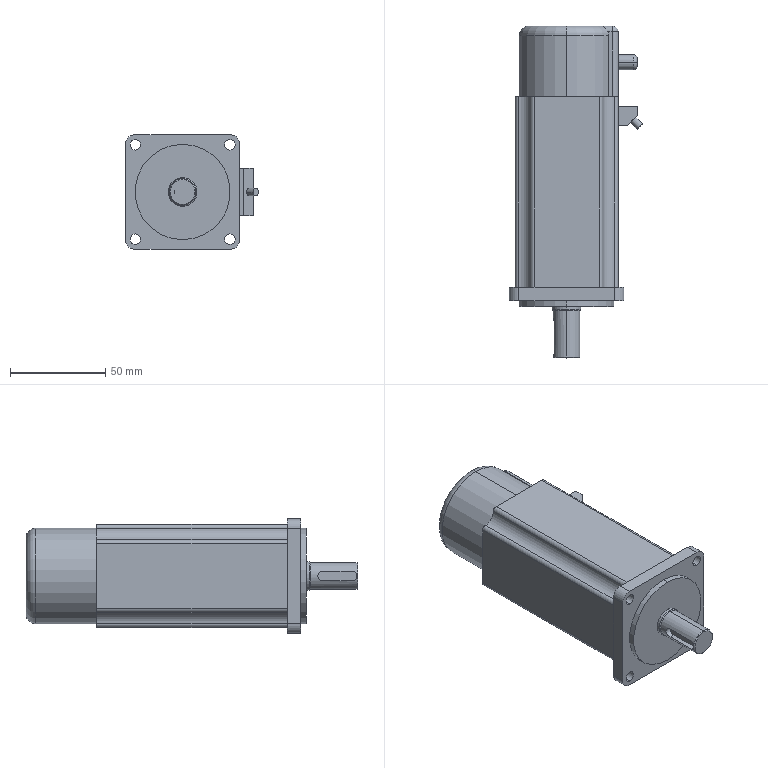Part | SolidWorks | features ICE 11, Fillet 6, Chamfer 2, Extrusion 1 | 1 solid | 82 faces | box 69.828 x 174 x 60 mm | volume 379758 mm3 | cylinder 44 | plane 27 | torus 7 | cone 2 | sphere 2 | commonest cylinder face diameters 4 x10 5.5 x8 6 x5 50 x5 10 x4 12 x4